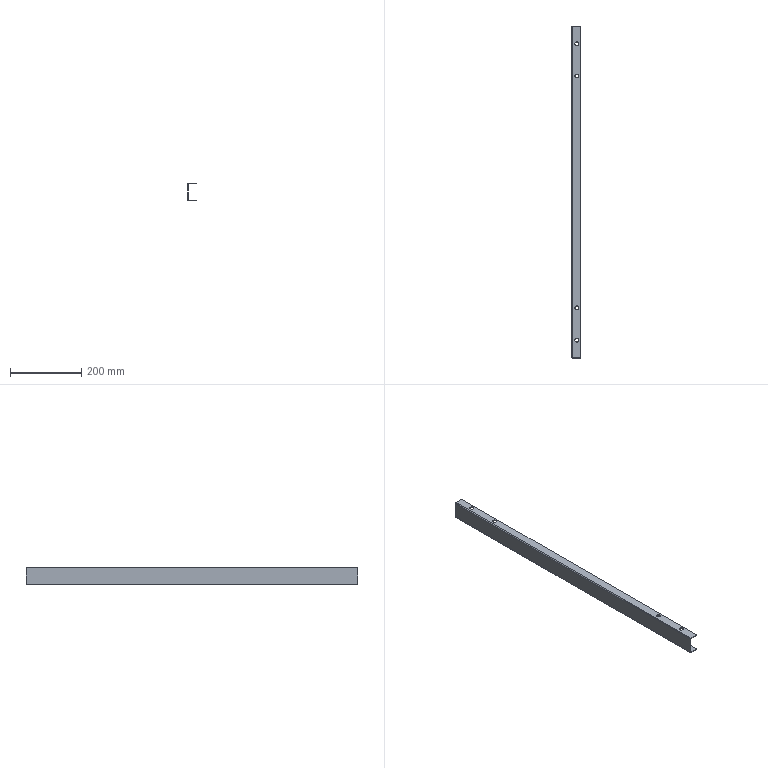Part | 1 solid | 38 faces | box 25 x 929 x 50 mm | volume 174934 mm3 | cylinder 20 | plane 18 | commonest cylinder face diameters 11 x16 0.4 x2 4.4 x2
STEP:
#1=CARTESIAN_POINT('',(20.5,414.5,-23.));
#2=VERTEX_POINT('',#1);
#3=CARTESIAN_POINT('',(9.5,414.5,-23.));
#4=VERTEX_POINT('',#3);
#5=CARTESIAN_POINT('',(15.,414.5,-23.));
#6=DIRECTION('',(0.,0.,-1.));
#7=DIRECTION('',(-1.,0.,0.));
#8=AXIS2_PLACEMENT_3D('',#5,#6,#7);
#9=CIRCLE('',#8,5.5);
#10=EDGE_CURVE('',#2,#4,#9,.T.);
#11=ORIENTED_EDGE('',*,*,#10,.F.);
#12=CARTESIAN_POINT('',(20.5,414.5,-25.));
#13=VERTEX_POINT('',#12);
#14=CARTESIAN_POINT('',(20.5,414.5,25.));
#15=DIRECTION('',(0.,0.,-1.));
#16=VECTOR('',#15,1000.);
#17=LINE('',#14,#16);
#18=EDGE_CURVE('',#2,#13,#17,.T.);
#19=ORIENTED_EDGE('',*,*,#18,.T.);
#20=CARTESIAN_POINT('',(9.5,414.5,-25.));
#21=VERTEX_POINT('',#20);
#22=CARTESIAN_POINT('',(15.,414.5,-25.));
#23=DIRECTION('',(0.,0.,-1.));
#24=DIRECTION('',(-1.,0.,0.));
#25=AXIS2_PLACEMENT_3D('',#22,#23,#24);
#26=CIRCLE('',#25,5.5);
#27=EDGE_CURVE('',#13,#21,#26,.T.);
#28=ORIENTED_EDGE('',*,*,#27,.T.);
#29=CARTESIAN_POINT('',(9.5,414.5,25.));
#30=DIRECTION('',(0.,0.,-1.));
#31=VECTOR('',#30,1000.);
#32=LINE('',#29,#31);
#33=EDGE_CURVE('',#4,#21,#32,.T.);
#34=ORIENTED_EDGE('',*,*,#33,.F.);
#35=EDGE_LOOP('',(#11,#19,#28,#34));
#36=FACE_OUTER_BOUND('',#35,.T.);
#37=CARTESIAN_POINT('',(15.,414.5,25.));
#38=DIRECTION('',(0.,0.,-1.));
#39=DIRECTION('',(-1.,0.,0.));
#40=AXIS2_PLACEMENT_3D('',#37,#38,#39);
#41=CYLINDRICAL_SURFACE('',#40,5.5);
#42=ADVANCED_FACE('',(#36),#41,.F.);
#43=CARTESIAN_POINT('',(20.5,324.5,-23.));
#44=VERTEX_POINT('',#43);
#45=CARTESIAN_POINT('',(9.5,324.5,-23.));
#46=VERTEX_POINT('',#45);
#47=CARTESIAN_POINT('',(15.,324.5,-23.));
#48=DIRECTION('',(0.,0.,-1.));
#49=DIRECTION('',(-1.,0.,0.));
#50=AXIS2_PLACEMENT_3D('',#47,#48,#49);
#51=CIRCLE('',#50,5.5);
#52=EDGE_CURVE('',#44,#46,#51,.T.);
#53=ORIENTED_EDGE('',*,*,#52,.F.);
#54=CARTESIAN_POINT('',(20.5,324.5,-25.));
#55=VERTEX_POINT('',#54);
#56=CARTESIAN_POINT('',(20.5,324.5,25.));
#57=DIRECTION('',(0.,0.,-1.));
#58=VECTOR('',#57,1000.);
#59=LINE('',#56,#58);
#60=EDGE_CURVE('',#44,#55,#59,.T.);
#61=ORIENTED_EDGE('',*,*,#60,.T.);
#62=CARTESIAN_POINT('',(9.5,324.5,-25.));
#63=VERTEX_POINT('',#62);
#64=CARTESIAN_POINT('',(15.,324.5,-25.));
#65=DIRECTION('',(0.,0.,-1.));
#66=DIRECTION('',(-1.,0.,0.));
#67=AXIS2_PLACEMENT_3D('',#64,#65,#66);
#68=CIRCLE('',#67,5.5);
#69=EDGE_CURVE('',#55,#63,#68,.T.);
#70=ORIENTED_EDGE('',*,*,#69,.T.);
#71=CARTESIAN_POINT('',(9.5,324.5,25.));
#72=DIRECTION('',(0.,0.,-1.));
#73=VECTOR('',#72,1000.);
#74=LINE('',#71,#73);
#75=EDGE_CURVE('',#46,#63,#74,.T.);
#76=ORIENTED_EDGE('',*,*,#75,.F.);
#77=EDGE_LOOP('',(#53,#61,#70,#76));
#78=FACE_OUTER_BOUND('',#77,.T.);
#79=CARTESIAN_POINT('',(15.,324.5,25.));
#80=DIRECTION('',(0.,0.,-1.));
#81=DIRECTION('',(-1.,0.,0.));
#82=AXIS2_PLACEMENT_3D('',#79,#80,#81);
#83=CYLINDRICAL_SURFACE('',#82,5.5);
#84=ADVANCED_FACE('',(#78),#83,.F.);
#85=CARTESIAN_POINT('',(20.5,-324.5,-23.));
#86=VERTEX_POINT('',#85);
#87=CARTESIAN_POINT('',(9.5,-324.5,-23.));
#88=VERTEX_POINT('',#87);
#89=CARTESIAN_POINT('',(15.,-324.5,-23.));
#90=DIRECTION('',(0.,0.,-1.));
#91=DIRECTION('',(-1.,0.,0.));
#92=AXIS2_PLACEMENT_3D('',#89,#90,#91);
#93=CIRCLE('',#92,5.5);
#94=EDGE_CURVE('',#86,#88,#93,.T.);
#95=ORIENTED_EDGE('',*,*,#94,.F.);
#96=CARTESIAN_POINT('',(20.5,-324.5,-25.));
#97=VERTEX_POINT('',#96);
#98=CARTESIAN_POINT('',(20.5,-324.5,25.));
#99=DIRECTION('',(0.,0.,-1.));
#100=VECTOR('',#99,1000.);
#101=LINE('',#98,#100);
#102=EDGE_CURVE('',#86,#97,#101,.T.);
#103=ORIENTED_EDGE('',*,*,#102,.T.);
#104=CARTESIAN_POINT('',(9.5,-324.5,-25.));
#105=VERTEX_POINT('',#104);
#106=CARTESIAN_POINT('',(15.,-324.5,-25.));
#107=DIRECTION('',(0.,0.,-1.));
#108=DIRECTION('',(-1.,0.,0.));
#109=AXIS2_PLACEMENT_3D('',#106,#107,#108);
#110=CIRCLE('',#109,5.5);
#111=EDGE_CURVE('',#97,#105,#110,.T.);
#112=ORIENTED_EDGE('',*,*,#111,.T.);
#113=CARTESIAN_POINT('',(9.5,-324.5,25.));
#114=DIRECTION('',(0.,0.,-1.));
#115=VECTOR('',#114,1000.);
#116=LINE('',#113,#115);
#117=EDGE_CURVE('',#88,#105,#116,.T.);
#118=ORIENTED_EDGE('',*,*,#117,.F.);
#119=EDGE_LOOP('',(#95,#103,#112,#118));
#120=FACE_OUTER_BOUND('',#119,.T.);
#121=CARTESIAN_POINT('',(15.,-324.5,25.));
#122=DIRECTION('',(0.,0.,-1.));
#123=DIRECTION('',(-1.,0.,0.));
#124=AXIS2_PLACEMENT_3D('',#121,#122,#123);
#125=CYLINDRICAL_SURFACE('',#124,5.5);
#126=ADVANCED_FACE('',(#120),#125,.F.);
#127=CARTESIAN_POINT('',(20.5,-414.5,-23.));
#128=VERTEX_POINT('',#127);
#129=CARTESIAN_POINT('',(9.5,-414.5,-23.));
#130=VERTEX_POINT('',#129);
#131=CARTESIAN_POINT('',(15.,-414.5,-23.));
#132=DIRECTION('',(0.,0.,-1.));
#133=DIRECTION('',(-1.,0.,0.));
#134=AXIS2_PLACEMENT_3D('',#131,#132,#133);
#135=CIRCLE('',#134,5.5);
#136=EDGE_CURVE('',#128,#130,#135,.T.);
#137=ORIENTED_EDGE('',*,*,#136,.F.);
#138=CARTESIAN_POINT('',(20.5,-414.5,-25.));
#139=VERTEX_POINT('',#138);
#140=CARTESIAN_POINT('',(20.5,-414.5,25.));
#141=DIRECTION('',(0.,0.,-1.));
#142=VECTOR('',#141,1000.);
#143=LINE('',#140,#142);
#144=EDGE_CURVE('',#128,#139,#143,.T.);
#145=ORIENTED_EDGE('',*,*,#144,.T.);
#146=CARTESIAN_POINT('',(9.5,-414.5,-25.));
#147=VERTEX_POINT('',#146);
#148=CARTESIAN_POINT('',(15.,-414.5,-25.));
#149=DIRECTION('',(0.,0.,-1.));
#150=DIRECTION('',(-1.,0.,0.));
#151=AXIS2_PLACEMENT_3D('',#148,#149,#150);
#152=CIRCLE('',#151,5.5);
#153=EDGE_CURVE('',#139,#147,#152,.T.);
#154=ORIENTED_EDGE('',*,*,#153,.T.);
#155=CARTESIAN_POINT('',(9.5,-414.5,25.));
#156=DIRECTION('',(0.,0.,-1.));
#157=VECTOR('',#156,1000.);
#158=LINE('',#155,#157);
#159=EDGE_CURVE('',#130,#147,#158,.T.);
#160=ORIENTED_EDGE('',*,*,#159,.F.);
#161=EDGE_LOOP('',(#137,#145,#154,#160));
#162=FACE_OUTER_BOUND('',#161,.T.);
#163=CARTESIAN_POINT('',(15.,-414.5,25.));
#164=DIRECTION('',(0.,0.,-1.));
#165=DIRECTION('',(-1.,0.,0.));
#166=AXIS2_PLACEMENT_3D('',#163,#164,#165);
#167=CYLINDRICAL_SURFACE('',#166,5.5);
#168=ADVANCED_FACE('',(#162),#167,.F.);
#169=CARTESIAN_POINT('',(20.5,414.5,25.));
#170=VERTEX_POINT('',#169);
#171=CARTESIAN_POINT('',(9.5,414.5,25.));
#172=VERTEX_POINT('',#171);
#173=CARTESIAN_POINT('',(15.,414.5,25.));
#174=DIRECTION('',(0.,0.,-1.));
#175=DIRECTION('',(-1.,0.,0.));
#176=AXIS2_PLACEMENT_3D('',#173,#174,#175);
#177=CIRCLE('',#176,5.5);
#178=EDGE_CURVE('',#170,#172,#177,.T.);
#179=ORIENTED_EDGE('',*,*,#178,.F.);
#180=CARTESIAN_POINT('',(20.5,414.5,23.));
#181=VERTEX_POINT('',#180);
#182=CARTESIAN_POINT('',(20.5,414.5,25.));
#183=DIRECTION('',(0.,0.,-1.));
#184=VECTOR('',#183,1000.);
#185=LINE('',#182,#184);
#186=EDGE_CURVE('',#170,#181,#185,.T.);
#187=ORIENTED_EDGE('',*,*,#186,.T.);
#188=CARTESIAN_POINT('',(9.5,414.5,23.));
#189=VERTEX_POINT('',#188);
#190=CARTESIAN_POINT('',(15.,414.5,23.));
#191=DIRECTION('',(0.,0.,1.));
#192=DIRECTION('',(1.,0.,0.));
#193=AXIS2_PLACEMENT_3D('',#190,#191,#192);
#194=CIRCLE('',#193,5.5);
#195=EDGE_CURVE('',#189,#181,#194,.T.);
#196=ORIENTED_EDGE('',*,*,#195,.F.);
#197=CARTESIAN_POINT('',(9.5,414.5,25.));
#198=DIRECTION('',(0.,0.,-1.));
#199=VECTOR('',#198,1000.);
#200=LINE('',#197,#199);
#201=EDGE_CURVE('',#172,#189,#200,.T.);
#202=ORIENTED_EDGE('',*,*,#201,.F.);
#203=EDGE_LOOP('',(#179,#187,#196,#202));
#204=FACE_OUTER_BOUND('',#203,.T.);
#205=CARTESIAN_POINT('',(15.,414.5,25.));
#206=DIRECTION('',(0.,0.,-1.));
#207=DIRECTION('',(-1.,0.,0.));
#208=AXIS2_PLACEMENT_3D('',#205,#206,#207);
#209=CYLINDRICAL_SURFACE('',#208,5.5);
#210=ADVANCED_FACE('',(#204),#209,.F.);
#211=CARTESIAN_POINT('',(20.5,324.5,25.));
#212=VERTEX_POINT('',#211);
#213=CARTESIAN_POINT('',(9.5,324.5,25.));
#214=VERTEX_POINT('',#213);
#215=CARTESIAN_POINT('',(15.,324.5,25.));
#216=DIRECTION('',(0.,0.,-1.));
#217=DIRECTION('',(-1.,0.,0.));
#218=AXIS2_PLACEMENT_3D('',#215,#216,#217);
#219=CIRCLE('',#218,5.5);
#220=EDGE_CURVE('',#212,#214,#219,.T.);
#221=ORIENTED_EDGE('',*,*,#220,.F.);
#222=CARTESIAN_POINT('',(20.5,324.5,23.));
#223=VERTEX_POINT('',#222);
#224=CARTESIAN_POINT('',(20.5,324.5,25.));
#225=DIRECTION('',(0.,0.,-1.));
#226=VECTOR('',#225,1000.);
#227=LINE('',#224,#226);
#228=EDGE_CURVE('',#212,#223,#227,.T.);
#229=ORIENTED_EDGE('',*,*,#228,.T.);
#230=CARTESIAN_POINT('',(9.5,324.5,23.));
#231=VERTEX_POINT('',#230);
#232=CARTESIAN_POINT('',(15.,324.5,23.));
#233=DIRECTION('',(0.,0.,1.));
#234=DIRECTION('',(1.,0.,0.));
#235=AXIS2_PLACEMENT_3D('',#232,#233,#234);
#236=CIRCLE('',#235,5.5);
#237=EDGE_CURVE('',#231,#223,#236,.T.);
#238=ORIENTED_EDGE('',*,*,#237,.F.);
#239=CARTESIAN_POINT('',(9.5,324.5,25.));
#240=DIRECTION('',(0.,0.,-1.));
#241=VECTOR('',#240,1000.);
#242=LINE('',#239,#241);
#243=EDGE_CURVE('',#214,#231,#242,.T.);
#244=ORIENTED_EDGE('',*,*,#243,.F.);
#245=EDGE_LOOP('',(#221,#229,#238,#244));
#246=FACE_OUTER_BOUND('',#245,.T.);
#247=CARTESIAN_POINT('',(15.,324.5,25.));
#248=DIRECTION('',(0.,0.,-1.));
#249=DIRECTION('',(-1.,0.,0.));
#250=AXIS2_PLACEMENT_3D('',#247,#248,#249);
#251=CYLINDRICAL_SURFACE('',#250,5.5);
#252=ADVANCED_FACE('',(#246),#251,.F.);
#253=CARTESIAN_POINT('',(20.5,-324.5,25.));
#254=VERTEX_POINT('',#253);
#255=CARTESIAN_POINT('',(9.5,-324.5,25.));
#256=VERTEX_POINT('',#255);
#257=CARTESIAN_POINT('',(15.,-324.5,25.));
#258=DIRECTION('',(0.,0.,-1.));
#259=DIRECTION('',(1.,0.,0.));
#260=AXIS2_PLACEMENT_3D('',#257,#258,#259);
#261=CIRCLE('',#260,5.5);
#262=EDGE_CURVE('',#254,#256,#261,.T.);
#263=ORIENTED_EDGE('',*,*,#262,.F.);
#264=CARTESIAN_POINT('',(20.5,-324.5,23.));
#265=VERTEX_POINT('',#264);
#266=CARTESIAN_POINT('',(20.5,-324.5,25.));
#267=DIRECTION('',(0.,0.,-1.));
#268=VECTOR('',#267,1000.);
#269=LINE('',#266,#268);
#270=EDGE_CURVE('',#254,#265,#269,.T.);
#271=ORIENTED_EDGE('',*,*,#270,.T.);
#272=CARTESIAN_POINT('',(9.5,-324.5,23.));
#273=VERTEX_POINT('',#272);
#274=CARTESIAN_POINT('',(15.,-324.5,23.));
#275=DIRECTION('',(0.,0.,1.));
#276=DIRECTION('',(1.,0.,0.));
#277=AXIS2_PLACEMENT_3D('',#274,#275,#276);
#278=CIRCLE('',#277,5.5);
#279=EDGE_CURVE('',#273,#265,#278,.T.);
#280=ORIENTED_EDGE('',*,*,#279,.F.);
#281=CARTESIAN_POINT('',(9.5,-324.5,25.));
#282=DIRECTION('',(0.,0.,-1.));
#283=VECTOR('',#282,1000.);
#284=LINE('',#281,#283);
#285=EDGE_CURVE('',#256,#273,#284,.T.);
#286=ORIENTED_EDGE('',*,*,#285,.F.);
#287=EDGE_LOOP('',(#263,#271,#280,#286));
#288=FACE_OUTER_BOUND('',#287,.T.);
#289=CARTESIAN_POINT('',(15.,-324.5,25.));
#290=DIRECTION('',(0.,0.,-1.));
#291=DIRECTION('',(-1.,0.,0.));
#292=AXIS2_PLACEMENT_3D('',#289,#290,#291);
#293=CYLINDRICAL_SURFACE('',#292,5.5);
#294=ADVANCED_FACE('',(#288),#293,.F.);
#295=CARTESIAN_POINT('',(20.5,-414.5,25.));
#296=VERTEX_POINT('',#295);
#297=CARTESIAN_POINT('',(9.5,-414.5,25.));
#298=VERTEX_POINT('',#297);
#299=CARTESIAN_POINT('',(15.,-414.5,25.));
#300=DIRECTION('',(0.,0.,-1.));
#301=DIRECTION('',(1.,0.,0.));
#302=AXIS2_PLACEMENT_3D('',#299,#300,#301);
#303=CIRCLE('',#302,5.5);
#304=EDGE_CURVE('',#296,#298,#303,.T.);
#305=ORIENTED_EDGE('',*,*,#304,.F.);
#306=CARTESIAN_POINT('',(20.5,-414.5,23.));
#307=VERTEX_POINT('',#306);
#308=CARTESIAN_POINT('',(20.5,-414.5,25.));
#309=DIRECTION('',(0.,0.,-1.));
#310=VECTOR('',#309,1000.);
#311=LINE('',#308,#310);
#312=EDGE_CURVE('',#296,#307,#311,.T.);
#313=ORIENTED_EDGE('',*,*,#312,.T.);
#314=CARTESIAN_POINT('',(9.5,-414.5,23.));
#315=VERTEX_POINT('',#314);
#316=CARTESIAN_POINT('',(15.,-414.5,23.));
#317=DIRECTION('',(0.,0.,1.));
#318=DIRECTION('',(1.,0.,0.));
#319=AXIS2_PLACEMENT_3D('',#316,#317,#318);
#320=CIRCLE('',#319,5.5);
#321=EDGE_CURVE('',#315,#307,#320,.T.);
#322=ORIENTED_EDGE('',*,*,#321,.F.);
#323=CARTESIAN_POINT('',(9.5,-414.5,25.));
#324=DIRECTION('',(0.,0.,-1.));
#325=VECTOR('',#324,1000.);
#326=LINE('',#323,#325);
#327=EDGE_CURVE('',#298,#315,#326,.T.);
#328=ORIENTED_EDGE('',*,*,#327,.F.);
#329=EDGE_LOOP('',(#305,#313,#322,#328));
#330=FACE_OUTER_BOUND('',#329,.T.);
#331=CARTESIAN_POINT('',(15.,-414.5,25.));
#332=DIRECTION('',(0.,0.,-1.));
#333=DIRECTION('',(-1.,0.,0.));
#334=AXIS2_PLACEMENT_3D('',#331,#332,#333);
#335=CYLINDRICAL_SURFACE('',#334,5.5);
#336=ADVANCED_FACE('',(#330),#335,.F.);
#337=CARTESIAN_POINT('',(0.,464.5,22.8));
#338=VERTEX_POINT('',#337);
#339=CARTESIAN_POINT('',(2.,464.5,22.8));
#340=VERTEX_POINT('',#339);
#341=CARTESIAN_POINT('',(0.,464.5,22.8));
#342=DIRECTION('',(1.,0.,0.));
#343=VECTOR('',#342,1000.);
#344=LINE('',#341,#343);
#345=EDGE_CURVE('',#338,#340,#344,.T.);
#346=ORIENTED_EDGE('',*,*,#345,.F.);
#347=CARTESIAN_POINT('',(2.2,464.5,25.));
#348=VERTEX_POINT('',#347);
#349=CARTESIAN_POINT('',(2.2,464.5,22.8));
#350=DIRECTION('',(0.,-1.,0.));
#351=DIRECTION('',(0.,0.,1.));
#352=AXIS2_PLACEMENT_3D('',#349,#350,#351);
#353=CIRCLE('',#352,2.2);
#354=EDGE_CURVE('',#348,#338,#353,.T.);
#355=ORIENTED_EDGE('',*,*,#354,.F.);
#356=CARTESIAN_POINT('',(2.2,464.5,23.));
#357=VERTEX_POINT('',#356);
#358=CARTESIAN_POINT('',(2.2,464.5,23.));
#359=DIRECTION('',(0.,0.,1.));
#360=VECTOR('',#359,1000.);
#361=LINE('',#358,#360);
#362=EDGE_CURVE('',#357,#348,#361,.T.);
#363=ORIENTED_EDGE('',*,*,#362,.F.);
#364=CARTESIAN_POINT('',(2.2,464.5,22.8));
#365=DIRECTION('',(0.,-1.,0.));
#366=DIRECTION('',(1.,0.,0.));
#367=AXIS2_PLACEMENT_3D('',#364,#365,#366);
#368=CIRCLE('',#367,0.2);
#369=EDGE_CURVE('',#357,#340,#368,.T.);
#370=ORIENTED_EDGE('',*,*,#369,.T.);
#371=EDGE_LOOP('',(#346,#355,#363,#370));
#372=FACE_OUTER_BOUND('',#371,.T.);
#373=CARTESIAN_POINT('',(0.,464.5,22.8));
#374=DIRECTION('',(0.,1.,0.));
#375=DIRECTION('',(0.,0.,1.));
#376=AXIS2_PLACEMENT_3D('',#373,#374,#375);
#377=PLANE('',#376);
#378=ADVANCED_FACE('',(#372),#377,.T.);
#379=CARTESIAN_POINT('',(0.,464.5,-22.8));
#380=VERTEX_POINT('',#379);
#381=CARTESIAN_POINT('',(0.,464.5,-25.));
#382=DIRECTION('',(0.,0.,-1.));
#383=VECTOR('',#382,1000.);
#384=LINE('',#381,#383);
#385=EDGE_CURVE('',#338,#380,#384,.T.);
#386=ORIENTED_EDGE('',*,*,#385,.F.);
#387=ORIENTED_EDGE('',*,*,#345,.T.);
#388=CARTESIAN_POINT('',(2.,464.5,-22.8));
#389=VERTEX_POINT('',#388);
#390=CARTESIAN_POINT('',(2.,464.5,-25.));
#391=DIRECTION('',(0.,0.,-1.));
#392=VECTOR('',#391,1000.);
#393=LINE('',#390,#392);
#394=EDGE_CURVE('',#340,#389,#393,.T.);
#395=ORIENTED_EDGE('',*,*,#394,.T.);
#396=CARTESIAN_POINT('',(2.,464.5,-22.8));
#397=DIRECTION('',(-1.,0.,0.));
#398=VECTOR('',#397,1000.);
#399=LINE('',#396,#398);
#400=EDGE_CURVE('',#389,#380,#399,.T.);
#401=ORIENTED_EDGE('',*,*,#400,.T.);
#402=EDGE_LOOP('',(#386,#387,#395,#401));
#403=FACE_OUTER_BOUND('',#402,.T.);
#404=CARTESIAN_POINT('',(2.2,464.5,23.));
#405=DIRECTION('',(0.,1.,0.));
#406=DIRECTION('',(0.,0.,1.));
#407=AXIS2_PLACEMENT_3D('',#404,#405,#406);
#408=PLANE('',#407);
#409=ADVANCED_FACE('',(#403),#408,.T.);
#410=CARTESIAN_POINT('',(2.2,-464.5,25.));
#411=VERTEX_POINT('',#410);
#412=CARTESIAN_POINT('',(2.2,-464.5,23.));
#413=VERTEX_POINT('',#412);
#414=CARTESIAN_POINT('',(2.2,-464.5,25.));
#415=DIRECTION('',(0.,0.,-1.));
#416=VECTOR('',#415,1000.);
#417=LINE('',#414,#416);
#418=EDGE_CURVE('',#411,#413,#417,.T.);
#419=ORIENTED_EDGE('',*,*,#418,.F.);
#420=CARTESIAN_POINT('',(0.,-464.5,22.8));
#421=VERTEX_POINT('',#420);
#422=CARTESIAN_POINT('',(2.2,-464.5,22.8));
#423=DIRECTION('',(0.,-1.,0.));
#424=DIRECTION('',(0.,0.,1.));
#425=AXIS2_PLACEMENT_3D('',#422,#423,#424);
#426=CIRCLE('',#425,2.2);
#427=EDGE_CURVE('',#411,#421,#426,.T.);
#428=ORIENTED_EDGE('',*,*,#427,.T.);
#429=CARTESIAN_POINT('',(2.,-464.5,22.8));
#430=VERTEX_POINT('',#429);
#431=CARTESIAN_POINT('',(2.,-464.5,22.8));
#432=DIRECTION('',(-1.,0.,0.));
#433=VECTOR('',#432,1000.);
#434=LINE('',#431,#433);
#435=EDGE_CURVE('',#430,#421,#434,.T.);
#436=ORIENTED_EDGE('',*,*,#435,.F.);
#437=CARTESIAN_POINT('',(2.2,-464.5,22.8));
#438=DIRECTION('',(0.,-1.,0.));
#439=DIRECTION('',(1.,0.,0.));
#440=AXIS2_PLACEMENT_3D('',#437,#438,#439);
#441=CIRCLE('',#440,0.2);
#442=EDGE_CURVE('',#413,#430,#441,.T.);
#443=ORIENTED_EDGE('',*,*,#442,.F.);
#444=EDGE_LOOP('',(#419,#428,#436,#443));
#445=FACE_OUTER_BOUND('',#444,.T.);
#446=CARTESIAN_POINT('',(2.2,-464.5,25.));
#447=DIRECTION('',(0.,-1.,0.));
#448=DIRECTION('',(0.,0.,-1.));
#449=AXIS2_PLACEMENT_3D('',#446,#447,#448);
#450=PLANE('',#449);
#451=ADVANCED_FACE('',(#445),#450,.T.);
#452=CARTESIAN_POINT('',(25.,-464.5,25.));
#453=VERTEX_POINT('',#452);
#454=CARTESIAN_POINT('',(0.,-464.5,25.));
#455=DIRECTION('',(-1.,0.,0.));
#456=VECTOR('',#455,1000.);
#457=LINE('',#454,#456);
#458=EDGE_CURVE('',#453,#411,#457,.T.);
#459=ORIENTED_EDGE('',*,*,#458,.T.);
#460=ORIENTED_EDGE('',*,*,#418,.T.);
#461=CARTESIAN_POINT('',(25.,-464.5,23.));
#462=VERTEX_POINT('',#461);
#463=CARTESIAN_POINT('',(0.,-464.5,23.));
#464=DIRECTION('',(-1.,0.,0.));
#465=VECTOR('',#464,1000.);
#466=LINE('',#463,#465);
#467=EDGE_CURVE('',#462,#413,#466,.T.);
#468=ORIENTED_EDGE('',*,*,#467,.F.);
#469=CARTESIAN_POINT('',(25.,-464.5,23.));
#470=DIRECTION('',(0.,0.,1.));
#471=VECTOR('',#470,1000.);
#472=LINE('',#469,#471);
#473=EDGE_CURVE('',#462,#453,#472,.T.);
#474=ORIENTED_EDGE('',*,*,#473,.T.);
#475=EDGE_LOOP('',(#459,#460,#468,#474));
#476=FACE_OUTER_BOUND('',#475,.T.);
#477=CARTESIAN_POINT('',(2.,-464.5,22.8));
#478=DIRECTION('',(0.,-1.,0.));
#479=DIRECTION('',(0.,0.,-1.));
#480=AXIS2_PLACEMENT_3D('',#477,#478,#479);
#481=PLANE('',#480);
#482=ADVANCED_FACE('',(#476),#481,.T.);
#483=CARTESIAN_POINT('',(2.2,464.5,-25.));
#484=VERTEX_POINT('',#483);
#485=CARTESIAN_POINT('',(2.2,464.5,-23.));
#486=VERTEX_POINT('',#485);
#487=CARTESIAN_POINT('',(2.2,464.5,-25.));
#488=DIRECTION('',(0.,0.,1.));
#489=VECTOR('',#488,1000.);
#490=LINE('',#487,#489);
#491=EDGE_CURVE('',#484,#486,#490,.T.);
#492=ORIENTED_EDGE('',*,*,#491,.F.);
#493=CARTESIAN_POINT('',(2.2,464.5,-22.8));
#494=DIRECTION('',(0.,-1.,0.));
#495=DIRECTION('',(0.,0.,1.));
#496=AXIS2_PLACEMENT_3D('',#493,#494,#495);
#497=CIRCLE('',#496,2.2);
#498=EDGE_CURVE('',#380,#484,#497,.T.);
#499=ORIENTED_EDGE('',*,*,#498,.F.);
#500=ORIENTED_EDGE('',*,*,#400,.F.);
#501=CARTESIAN_POINT('',(2.2,464.5,-22.8));
#502=DIRECTION('',(0.,-1.,0.));
#503=DIRECTION('',(1.,0.,0.));
#504=AXIS2_PLACEMENT_3D('',#501,#502,#503);
#505=CIRCLE('',#504,0.2);
#506=EDGE_CURVE('',#389,#486,#505,.T.);
#507=ORIENTED_EDGE('',*,*,#506,.T.);
#508=EDGE_LOOP('',(#492,#499,#500,#507));
#509=FACE_OUTER_BOUND('',#508,.T.);
#510=CARTESIAN_POINT('',(2.2,464.5,-25.));
#511=DIRECTION('',(0.,1.,0.));
#512=DIRECTION('',(0.,0.,1.));
#513=AXIS2_PLACEMENT_3D('',#510,#511,#512);
#514=PLANE('',#513);
#515=ADVANCED_FACE('',(#509),#514,.T.);
#516=CARTESIAN_POINT('',(25.,464.5,-25.));
#517=VERTEX_POINT('',#516);
#518=CARTESIAN_POINT('',(0.,464.5,-25.));
#519=DIRECTION('',(1.,0.,0.));
#520=VECTOR('',#519,1000.);
#521=LINE('',#518,#520);
#522=EDGE_CURVE('',#484,#517,#521,.T.);
#523=ORIENTED_EDGE('',*,*,#522,.F.);
#524=ORIENTED_EDGE('',*,*,#491,.T.);
#525=CARTESIAN_POINT('',(25.,464.5,-23.));
#526=VERTEX_POINT('',#525);
#527=CARTESIAN_POINT('',(0.,464.5,-23.));
#528=DIRECTION('',(1.,0.,0.));
#529=VECTOR('',#528,1000.);
#530=LINE('',#527,#529);
#531=EDGE_CURVE('',#486,#526,#530,.T.);
#532=ORIENTED_EDGE('',*,*,#531,.T.);
#533=CARTESIAN_POINT('',(25.,464.5,-25.));
#534=DIRECTION('',(0.,0.,1.));
#535=VECTOR('',#534,1000.);
#536=LINE('',#533,#535);
#537=EDGE_CURVE('',#517,#526,#536,.T.);
#538=ORIENTED_EDGE('',*,*,#537,.F.);
#539=EDGE_LOOP('',(#523,#524,#532,#538));
#540=FACE_OUTER_BOUND('',#539,.T.);
#541=CARTESIAN_POINT('',(2.,464.5,-22.8));
#542=DIRECTION('',(0.,1.,0.));
#543=DIRECTION('',(0.,0.,1.));
#544=AXIS2_PLACEMENT_3D('',#541,#542,#543);
#545=PLANE('',#544);
#546=ADVANCED_FACE('',(#540),#545,.T.);
#547=CARTESIAN_POINT('',(0.,-464.5,-22.8));
#548=VERTEX_POINT('',#547);
#549=CARTESIAN_POINT('',(2.,-464.5,-22.8));
#550=VERTEX_POINT('',#549);
#551=CARTESIAN_POINT('',(0.,-464.5,-22.8));
#552=DIRECTION('',(1.,0.,0.));
#553=VECTOR('',#552,1000.);
#554=LINE('',#551,#553);
#555=EDGE_CURVE('',#548,#550,#554,.T.);
#556=ORIENTED_EDGE('',*,*,#555,.F.);
#557=CARTESIAN_POINT('',(2.2,-464.5,-25.));
#558=VERTEX_POINT('',#557);
#559=CARTESIAN_POINT('',(2.2,-464.5,-22.8));
#560=DIRECTION('',(0.,-1.,0.));
#561=DIRECTION('',(0.,0.,1.));
#562=AXIS2_PLACEMENT_3D('',#559,#560,#561);
#563=CIRCLE('',#562,2.2);
#564=EDGE_CURVE('',#548,#558,#563,.T.);
#565=ORIENTED_EDGE('',*,*,#564,.T.);
#566=CARTESIAN_POINT('',(2.2,-464.5,-23.));
#567=VERTEX_POINT('',#566);
#568=CARTESIAN_POINT('',(2.2,-464.5,-23.));
#569=DIRECTION('',(0.,0.,-1.));
#570=VECTOR('',#569,1000.);
#571=LINE('',#568,#570);
#572=EDGE_CURVE('',#567,#558,#571,.T.);
#573=ORIENTED_EDGE('',*,*,#572,.F.);
#574=CARTESIAN_POINT('',(2.2,-464.5,-22.8));
#575=DIRECTION('',(0.,-1.,0.));
#576=DIRECTION('',(1.,0.,0.));
#577=AXIS2_PLACEMENT_3D('',#574,#575,#576);
#578=CIRCLE('',#577,0.2);
#579=EDGE_CURVE('',#550,#567,#578,.T.);
#580=ORIENTED_EDGE('',*,*,#579,.F.);
#581=EDGE_LOOP('',(#556,#565,#573,#580));
#582=FACE_OUTER_BOUND('',#581,.T.);
#583=CARTESIAN_POINT('',(0.,-464.5,-22.8));
#584=DIRECTION('',(0.,-1.,0.));
#585=DIRECTION('',(0.,0.,-1.));
#586=AXIS2_PLACEMENT_3D('',#583,#584,#585);
#587=PLANE('',#586);
#588=ADVANCED_FACE('',(#582),#587,.T.);
#589=CARTESIAN_POINT('',(0.,-464.5,-25.));
#590=DIRECTION('',(0.,0.,-1.));
#591=VECTOR('',#590,1000.);
#592=LINE('',#589,#591);
#593=EDGE_CURVE('',#421,#548,#592,.T.);
#594=ORIENTED_EDGE('',*,*,#593,.T.);
#595=ORIENTED_EDGE('',*,*,#555,.T.);
#596=CARTESIAN_POINT('',(2.,-464.5,-25.));
#597=DIRECTION('',(0.,0.,-1.));
#598=VECTOR('',#597,1000.);
#599=LINE('',#596,#598);
#600=EDGE_CURVE('',#430,#550,#599,.T.);
#601=ORIENTED_EDGE('',*,*,#600,.F.);
#602=ORIENTED_EDGE('',*,*,#435,.T.);
#603=EDGE_LOOP('',(#594,#595,#601,#602));
#604=FACE_OUTER_BOUND('',#603,.T.);
#605=CARTESIAN_POINT('',(2.2,-464.5,-23.));
#606=DIRECTION('',(0.,-1.,0.));
#607=DIRECTION('',(0.,0.,-1.));
#608=AXIS2_PLACEMENT_3D('',#605,#606,#607);
#609=PLANE('',#608);
#610=ADVANCED_FACE('',(#604),#609,.T.);
#611=CARTESIAN_POINT('',(15.,414.5,-23.));
#612=DIRECTION('',(0.,0.,-1.));
#613=DIRECTION('',(-1.,0.,0.));
#614=AXIS2_PLACEMENT_3D('',#611,#612,#613);
#615=CIRCLE('',#614,5.5);
#616=EDGE_CURVE('',#4,#2,#615,.T.);
#617=ORIENTED_EDGE('',*,*,#616,.T.);
#618=ORIENTED_EDGE('',*,*,#10,.T.);
#619=EDGE_LOOP('',(#617,#618));
#620=FACE_BOUND('',#619,.T.);
#621=CARTESIAN_POINT('',(15.,324.5,-23.));
#622=DIRECTION('',(0.,0.,-1.));
#623=DIRECTION('',(-1.,0.,0.));
#624=AXIS2_PLACEMENT_3D('',#621,#622,#623);
#625=CIRCLE('',#624,5.5);
#626=EDGE_CURVE('',#46,#44,#625,.T.);
#627=ORIENTED_EDGE('',*,*,#626,.T.);
#628=ORIENTED_EDGE('',*,*,#52,.T.);
#629=EDGE_LOOP('',(#627,#628));
#630=FACE_BOUND('',#629,.T.);
#631=CARTESIAN_POINT('',(15.,-324.5,-23.));
#632=DIRECTION('',(0.,0.,-1.));
#633=DIRECTION('',(-1.,0.,0.));
#634=AXIS2_PLACEMENT_3D('',#631,#632,#633);
#635=CIRCLE('',#634,5.5);
#636=EDGE_CURVE('',#88,#86,#635,.T.);
#637=ORIENTED_EDGE('',*,*,#636,.T.);
#638=ORIENTED_EDGE('',*,*,#94,.T.);
#639=EDGE_LOOP('',(#637,#638));
#640=FACE_BOUND('',#639,.T.);
#641=CARTESIAN_POINT('',(15.,-414.5,-23.));
#642=DIRECTION('',(0.,0.,-1.));
#643=DIRECTION('',(-1.,0.,0.));
#644=AXIS2_PLACEMENT_3D('',#641,#642,#643);
#645=CIRCLE('',#644,5.5);
#646=EDGE_CURVE('',#130,#128,#645,.T.);
#647=ORIENTED_EDGE('',*,*,#646,.T.);
#648=ORIENTED_EDGE('',*,*,#136,.T.);
#649=EDGE_LOOP('',(#647,#648));
#650=FACE_BOUND('',#649,.T.);
#651=CARTESIAN_POINT('',(25.,-464.5,-23.));
#652=VERTEX_POINT('',#651);
#653=CARTESIAN_POINT('',(0.,-464.5,-23.));
#654=DIRECTION('',(1.,0.,0.));
#655=VECTOR('',#654,1000.);
#656=LINE('',#653,#655);
#657=EDGE_CURVE('',#567,#652,#656,.T.);
#658=ORIENTED_EDGE('',*,*,#657,.T.);
#659=CARTESIAN_POINT('',(25.,464.5,-23.));
#660=DIRECTION('',(0.,-1.,0.));
#661=VECTOR('',#660,1000.);
#662=LINE('',#659,#661);
#663=EDGE_CURVE('',#526,#652,#662,.T.);
#664=ORIENTED_EDGE('',*,*,#663,.F.);
#665=ORIENTED_EDGE('',*,*,#531,.F.);
#666=CARTESIAN_POINT('',(2.2,464.5,-23.));
#667=DIRECTION('',(0.,-1.,0.));
#668=VECTOR('',#667,1000.);
#669=LINE('',#666,#668);
#670=EDGE_CURVE('',#486,#567,#669,.T.);
#671=ORIENTED_EDGE('',*,*,#670,.T.);
#672=EDGE_LOOP('',(#658,#664,#665,#671));
#673=FACE_OUTER_BOUND('',#672,.T.);
#674=CARTESIAN_POINT('',(0.,464.5,-23.));
#675=DIRECTION('',(0.,0.,-1.));
#676=DIRECTION('',(-1.,0.,0.));
#677=AXIS2_PLACEMENT_3D('',#674,#675,#676);
#678=PLANE('',#677);
#679=ADVANCED_FACE('',(#620,#630,#640,#650,#673),#678,.F.);
#680=CARTESIAN_POINT('',(25.,-464.5,-25.));
#681=VERTEX_POINT('',#680);
#682=CARTESIAN_POINT('',(25.,-464.5,-25.));
#683=DIRECTION('',(0.,0.,1.));
#684=VECTOR('',#683,1000.);
#685=LINE('',#682,#684);
#686=EDGE_CURVE('',#681,#652,#685,.T.);
#687=ORIENTED_EDGE('',*,*,#686,.F.);
#688=CARTESIAN_POINT('',(25.,464.5,-25.));
#689=DIRECTION('',(0.,-1.,0.));
#690=VECTOR('',#689,1000.);
#691=LINE('',#688,#690);
#692=EDGE_CURVE('',#517,#681,#691,.T.);
#693=ORIENTED_EDGE('',*,*,#692,.F.);
#694=ORIENTED_EDGE('',*,*,#537,.T.);
#695=ORIENTED_EDGE('',*,*,#663,.T.);
#696=EDGE_LOOP('',(#687,#693,#694,#695));
#697=FACE_OUTER_BOUND('',#696,.T.);
#698=CARTESIAN_POINT('',(25.,464.5,-25.));
#699=DIRECTION('',(1.,0.,0.));
#700=DIRECTION('',(0.,0.,-1.));
#701=AXIS2_PLACEMENT_3D('',#698,#699,#700);
#702=PLANE('',#701);
#703=ADVANCED_FACE('',(#697),#702,.T.);
#704=CARTESIAN_POINT('',(15.,414.5,-25.));
#705=DIRECTION('',(0.,0.,-1.));
#706=DIRECTION('',(-1.,0.,0.));
#707=AXIS2_PLACEMENT_3D('',#704,#705,#706);
#708=CIRCLE('',#707,5.5);
#709=EDGE_CURVE('',#21,#13,#708,.T.);
#710=ORIENTED_EDGE('',*,*,#709,.F.);
#711=ORIENTED_EDGE('',*,*,#27,.F.);
#712=EDGE_LOOP('',(#710,#711));
#713=FACE_BOUND('',#712,.T.);
#714=CARTESIAN_POINT('',(15.,324.5,-25.));
#715=DIRECTION('',(0.,0.,-1.));
#716=DIRECTION('',(-1.,0.,0.));
#717=AXIS2_PLACEMENT_3D('',#714,#715,#716);
#718=CIRCLE('',#717,5.5);
#719=EDGE_CURVE('',#63,#55,#718,.T.);
#720=ORIENTED_EDGE('',*,*,#719,.F.);
#721=ORIENTED_EDGE('',*,*,#69,.F.);
#722=EDGE_LOOP('',(#720,#721));
#723=FACE_BOUND('',#722,.T.);
#724=CARTESIAN_POINT('',(15.,-324.5,-25.));
#725=DIRECTION('',(0.,0.,-1.));
#726=DIRECTION('',(-1.,0.,0.));
#727=AXIS2_PLACEMENT_3D('',#724,#725,#726);
#728=CIRCLE('',#727,5.5);
#729=EDGE_CURVE('',#105,#97,#728,.T.);
#730=ORIENTED_EDGE('',*,*,#729,.F.);
#731=ORIENTED_EDGE('',*,*,#111,.F.);
#732=EDGE_LOOP('',(#730,#731));
#733=FACE_BOUND('',#732,.T.);
#734=CARTESIAN_POINT('',(15.,-414.5,-25.));
#735=DIRECTION('',(0.,0.,-1.));
#736=DIRECTION('',(-1.,0.,0.));
#737=AXIS2_PLACEMENT_3D('',#734,#735,#736);
#738=CIRCLE('',#737,5.5);
#739=EDGE_CURVE('',#147,#139,#738,.T.);
#740=ORIENTED_EDGE('',*,*,#739,.F.);
#741=ORIENTED_EDGE('',*,*,#153,.F.);
#742=EDGE_LOOP('',(#740,#741));
#743=FACE_BOUND('',#742,.T.);
#744=CARTESIAN_POINT('',(0.,-464.5,-25.));
#745=DIRECTION('',(1.,0.,0.));
#746=VECTOR('',#745,1000.);
#747=LINE('',#744,#746);
#748=EDGE_CURVE('',#558,#681,#747,.T.);
#749=ORIENTED_EDGE('',*,*,#748,.F.);
#750=CARTESIAN_POINT('',(2.2,464.5,-25.));
#751=DIRECTION('',(0.,-1.,0.));
#752=VECTOR('',#751,1000.);
#753=LINE('',#750,#752);
#754=EDGE_CURVE('',#484,#558,#753,.T.);
#755=ORIENTED_EDGE('',*,*,#754,.F.);
#756=ORIENTED_EDGE('',*,*,#522,.T.);
#757=ORIENTED_EDGE('',*,*,#692,.T.);
#758=EDGE_LOOP('',(#749,#755,#756,#757));
#759=FACE_OUTER_BOUND('',#758,.T.);
#760=CARTESIAN_POINT('',(0.,464.5,-25.));
#761=DIRECTION('',(0.,0.,-1.));
#762=DIRECTION('',(-1.,0.,0.));
#763=AXIS2_PLACEMENT_3D('',#760,#761,#762);
#764=PLANE('',#763);
#765=ADVANCED_FACE('',(#713,#723,#733,#743,#759),#764,.T.);
#766=ORIENTED_EDGE('',*,*,#564,.F.);
#767=CARTESIAN_POINT('',(0.,464.5,-22.8));
#768=DIRECTION('',(0.,-1.,0.));
#769=VECTOR('',#768,1000.);
#770=LINE('',#767,#769);
#771=EDGE_CURVE('',#380,#548,#770,.T.);
#772=ORIENTED_EDGE('',*,*,#771,.F.);
#773=ORIENTED_EDGE('',*,*,#498,.T.);
#774=ORIENTED_EDGE('',*,*,#754,.T.);
#775=EDGE_LOOP('',(#766,#772,#773,#774));
#776=FACE_OUTER_BOUND('',#775,.T.);
#777=CARTESIAN_POINT('',(2.2,464.5,-22.8));
#778=DIRECTION('',(0.,-1.,0.));
#779=DIRECTION('',(0.,0.,-1.));
#780=AXIS2_PLACEMENT_3D('',#777,#778,#779);
#781=CYLINDRICAL_SURFACE('',#780,2.2);
#782=ADVANCED_FACE('',(#776),#781,.T.);
#783=ORIENTED_EDGE('',*,*,#593,.F.);
#784=CARTESIAN_POINT('',(0.,464.5,22.8));
#785=DIRECTION('',(0.,-1.,0.));
#786=VECTOR('',#785,1000.);
#787=LINE('',#784,#786);
#788=EDGE_CURVE('',#338,#421,#787,.T.);
#789=ORIENTED_EDGE('',*,*,#788,.F.);
#790=ORIENTED_EDGE('',*,*,#385,.T.);
#791=ORIENTED_EDGE('',*,*,#771,.T.);
#792=EDGE_LOOP('',(#783,#789,#790,#791));
#793=FACE_OUTER_BOUND('',#792,.T.);
#794=CARTESIAN_POINT('',(0.,464.5,-25.));
#795=DIRECTION('',(-1.,0.,0.));
#796=DIRECTION('',(0.,0.,1.));
#797=AXIS2_PLACEMENT_3D('',#794,#795,#796);
#798=PLANE('',#797);
#799=ADVANCED_FACE('',(#793),#798,.T.);
#800=ORIENTED_EDGE('',*,*,#427,.F.);
#801=CARTESIAN_POINT('',(2.2,464.5,25.));
#802=DIRECTION('',(0.,-1.,0.));
#803=VECTOR('',#802,1000.);
#804=LINE('',#801,#803);
#805=EDGE_CURVE('',#348,#411,#804,.T.);
#806=ORIENTED_EDGE('',*,*,#805,.F.);
#807=ORIENTED_EDGE('',*,*,#354,.T.);
#808=ORIENTED_EDGE('',*,*,#788,.T.);
#809=EDGE_LOOP('',(#800,#806,#807,#808));
#810=FACE_OUTER_BOUND('',#809,.T.);
#811=CARTESIAN_POINT('',(2.2,464.5,22.8));
#812=DIRECTION('',(0.,-1.,0.));
#813=DIRECTION('',(0.,0.,-1.));
#814=AXIS2_PLACEMENT_3D('',#811,#812,#813);
#815=CYLINDRICAL_SURFACE('',#814,2.2);
#816=ADVANCED_FACE('',(#810),#815,.T.);
#817=CARTESIAN_POINT('',(15.,414.5,25.));
#818=DIRECTION('',(0.,0.,-1.));
#819=DIRECTION('',(-1.,0.,0.));
#820=AXIS2_PLACEMENT_3D('',#817,#818,#819);
#821=CIRCLE('',#820,5.5);
#822=EDGE_CURVE('',#172,#170,#821,.T.);
#823=ORIENTED_EDGE('',*,*,#822,.T.);
#824=ORIENTED_EDGE('',*,*,#178,.T.);
#825=EDGE_LOOP('',(#823,#824));
#826=FACE_BOUND('',#825,.T.);
#827=CARTESIAN_POINT('',(15.,324.5,25.));
#828=DIRECTION('',(0.,0.,-1.));
#829=DIRECTION('',(-1.,0.,0.));
#830=AXIS2_PLACEMENT_3D('',#827,#828,#829);
#831=CIRCLE('',#830,5.5);
#832=EDGE_CURVE('',#214,#212,#831,.T.);
#833=ORIENTED_EDGE('',*,*,#832,.T.);
#834=ORIENTED_EDGE('',*,*,#220,.T.);
#835=EDGE_LOOP('',(#833,#834));
#836=FACE_BOUND('',#835,.T.);
#837=CARTESIAN_POINT('',(15.,-324.5,25.));
#838=DIRECTION('',(0.,0.,-1.));
#839=DIRECTION('',(1.,0.,0.));
#840=AXIS2_PLACEMENT_3D('',#837,#838,#839);
#841=CIRCLE('',#840,5.5);
#842=EDGE_CURVE('',#256,#254,#841,.T.);
#843=ORIENTED_EDGE('',*,*,#842,.T.);
#844=ORIENTED_EDGE('',*,*,#262,.T.);
#845=EDGE_LOOP('',(#843,#844));
#846=FACE_BOUND('',#845,.T.);
#847=CARTESIAN_POINT('',(15.,-414.5,25.));
#848=DIRECTION('',(0.,0.,-1.));
#849=DIRECTION('',(1.,0.,0.));
#850=AXIS2_PLACEMENT_3D('',#847,#848,#849);
#851=CIRCLE('',#850,5.5);
#852=EDGE_CURVE('',#298,#296,#851,.T.);
#853=ORIENTED_EDGE('',*,*,#852,.T.);
#854=ORIENTED_EDGE('',*,*,#304,.T.);
#855=EDGE_LOOP('',(#853,#854));
#856=FACE_BOUND('',#855,.T.);
#857=ORIENTED_EDGE('',*,*,#458,.F.);
#858=CARTESIAN_POINT('',(25.,464.5,25.));
#859=VERTEX_POINT('',#858);
#860=CARTESIAN_POINT('',(25.,464.5,25.));
#861=DIRECTION('',(0.,-1.,0.));
#862=VECTOR('',#861,1000.);
#863=LINE('',#860,#862);
#864=EDGE_CURVE('',#859,#453,#863,.T.);
#865=ORIENTED_EDGE('',*,*,#864,.F.);
#866=CARTESIAN_POINT('',(0.,464.5,25.));
#867=DIRECTION('',(-1.,0.,0.));
#868=VECTOR('',#867,1000.);
#869=LINE('',#866,#868);
#870=EDGE_CURVE('',#859,#348,#869,.T.);
#871=ORIENTED_EDGE('',*,*,#870,.T.);
#872=ORIENTED_EDGE('',*,*,#805,.T.);
#873=EDGE_LOOP('',(#857,#865,#871,#872));
#874=FACE_OUTER_BOUND('',#873,.T.);
#875=CARTESIAN_POINT('',(0.,464.5,25.));
#876=DIRECTION('',(0.,0.,1.));
#877=DIRECTION('',(1.,0.,0.));
#878=AXIS2_PLACEMENT_3D('',#875,#876,#877);
#879=PLANE('',#878);
#880=ADVANCED_FACE('',(#826,#836,#846,#856,#874),#879,.T.);
#881=ORIENTED_EDGE('',*,*,#473,.F.);
#882=CARTESIAN_POINT('',(25.,464.5,23.));
#883=VERTEX_POINT('',#882);
#884=CARTESIAN_POINT('',(25.,464.5,23.));
#885=DIRECTION('',(0.,-1.,0.));
#886=VECTOR('',#885,1000.);
#887=LINE('',#884,#886);
#888=EDGE_CURVE('',#883,#462,#887,.T.);
#889=ORIENTED_EDGE('',*,*,#888,.F.);
#890=CARTESIAN_POINT('',(25.,464.5,23.));
#891=DIRECTION('',(0.,0.,1.));
#892=VECTOR('',#891,1000.);
#893=LINE('',#890,#892);
#894=EDGE_CURVE('',#883,#859,#893,.T.);
#895=ORIENTED_EDGE('',*,*,#894,.T.);
#896=ORIENTED_EDGE('',*,*,#864,.T.);
#897=EDGE_LOOP('',(#881,#889,#895,#896));
#898=FACE_OUTER_BOUND('',#897,.T.);
#899=CARTESIAN_POINT('',(25.,464.5,23.));
#900=DIRECTION('',(1.,0.,0.));
#901=DIRECTION('',(0.,0.,-1.));
#902=AXIS2_PLACEMENT_3D('',#899,#900,#901);
#903=PLANE('',#902);
#904=ADVANCED_FACE('',(#898),#903,.T.);
#905=ORIENTED_EDGE('',*,*,#195,.T.);
#906=CARTESIAN_POINT('',(15.,414.5,23.));
#907=DIRECTION('',(0.,0.,1.));
#908=DIRECTION('',(1.,0.,0.));
#909=AXIS2_PLACEMENT_3D('',#906,#907,#908);
#910=CIRCLE('',#909,5.5);
#911=EDGE_CURVE('',#181,#189,#910,.T.);
#912=ORIENTED_EDGE('',*,*,#911,.T.);
#913=EDGE_LOOP('',(#905,#912));
#914=FACE_BOUND('',#913,.T.);
#915=ORIENTED_EDGE('',*,*,#237,.T.);
#916=CARTESIAN_POINT('',(15.,324.5,23.));
#917=DIRECTION('',(0.,0.,1.));
#918=DIRECTION('',(1.,0.,0.));
#919=AXIS2_PLACEMENT_3D('',#916,#917,#918);
#920=CIRCLE('',#919,5.5);
#921=EDGE_CURVE('',#223,#231,#920,.T.);
#922=ORIENTED_EDGE('',*,*,#921,.T.);
#923=EDGE_LOOP('',(#915,#922));
#924=FACE_BOUND('',#923,.T.);
#925=ORIENTED_EDGE('',*,*,#279,.T.);
#926=CARTESIAN_POINT('',(15.,-324.5,23.));
#927=DIRECTION('',(0.,0.,1.));
#928=DIRECTION('',(1.,0.,0.));
#929=AXIS2_PLACEMENT_3D('',#926,#927,#928);
#930=CIRCLE('',#929,5.5);
#931=EDGE_CURVE('',#265,#273,#930,.T.);
#932=ORIENTED_EDGE('',*,*,#931,.T.);
#933=EDGE_LOOP('',(#925,#932));
#934=FACE_BOUND('',#933,.T.);
#935=ORIENTED_EDGE('',*,*,#321,.T.);
#936=CARTESIAN_POINT('',(15.,-414.5,23.));
#937=DIRECTION('',(0.,0.,1.));
#938=DIRECTION('',(1.,0.,0.));
#939=AXIS2_PLACEMENT_3D('',#936,#937,#938);
#940=CIRCLE('',#939,5.5);
#941=EDGE_CURVE('',#307,#315,#940,.T.);
#942=ORIENTED_EDGE('',*,*,#941,.T.);
#943=EDGE_LOOP('',(#935,#942));
#944=FACE_BOUND('',#943,.T.);
#945=ORIENTED_EDGE('',*,*,#467,.T.);
#946=CARTESIAN_POINT('',(2.2,464.5,23.));
#947=DIRECTION('',(0.,-1.,0.));
#948=VECTOR('',#947,1000.);
#949=LINE('',#946,#948);
#950=EDGE_CURVE('',#357,#413,#949,.T.);
#951=ORIENTED_EDGE('',*,*,#950,.F.);
#952=CARTESIAN_POINT('',(0.,464.5,23.));
#953=DIRECTION('',(-1.,0.,0.));
#954=VECTOR('',#953,1000.);
#955=LINE('',#952,#954);
#956=EDGE_CURVE('',#883,#357,#955,.T.);
#957=ORIENTED_EDGE('',*,*,#956,.F.);
#958=ORIENTED_EDGE('',*,*,#888,.T.);
#959=EDGE_LOOP('',(#945,#951,#957,#958));
#960=FACE_OUTER_BOUND('',#959,.T.);
#961=CARTESIAN_POINT('',(0.,464.5,23.));
#962=DIRECTION('',(0.,0.,1.));
#963=DIRECTION('',(1.,0.,0.));
#964=AXIS2_PLACEMENT_3D('',#961,#962,#963);
#965=PLANE('',#964);
#966=ADVANCED_FACE('',(#914,#924,#934,#944,#960),#965,.F.);
#967=ORIENTED_EDGE('',*,*,#442,.T.);
#968=CARTESIAN_POINT('',(2.,464.5,22.8));
#969=DIRECTION('',(0.,-1.,0.));
#970=VECTOR('',#969,1000.);
#971=LINE('',#968,#970);
#972=EDGE_CURVE('',#340,#430,#971,.T.);
#973=ORIENTED_EDGE('',*,*,#972,.F.);
#974=ORIENTED_EDGE('',*,*,#369,.F.);
#975=ORIENTED_EDGE('',*,*,#950,.T.);
#976=EDGE_LOOP('',(#967,#973,#974,#975));
#977=FACE_OUTER_BOUND('',#976,.T.);
#978=CARTESIAN_POINT('',(2.2,464.5,22.8));
#979=DIRECTION('',(0.,-1.,0.));
#980=DIRECTION('',(0.,0.,-1.));
#981=AXIS2_PLACEMENT_3D('',#978,#979,#980);
#982=CYLINDRICAL_SURFACE('',#981,0.2);
#983=ADVANCED_FACE('',(#977),#982,.F.);
#984=ORIENTED_EDGE('',*,*,#600,.T.);
#985=CARTESIAN_POINT('',(2.,464.5,-22.8));
#986=DIRECTION('',(0.,-1.,0.));
#987=VECTOR('',#986,1000.);
#988=LINE('',#985,#987);
#989=EDGE_CURVE('',#389,#550,#988,.T.);
#990=ORIENTED_EDGE('',*,*,#989,.F.);
#991=ORIENTED_EDGE('',*,*,#394,.F.);
#992=ORIENTED_EDGE('',*,*,#972,.T.);
#993=EDGE_LOOP('',(#984,#990,#991,#992));
#994=FACE_OUTER_BOUND('',#993,.T.);
#995=CARTESIAN_POINT('',(2.,464.5,-25.));
#996=DIRECTION('',(-1.,0.,0.));
#997=DIRECTION('',(0.,0.,1.));
#998=AXIS2_PLACEMENT_3D('',#995,#996,#997);
#999=PLANE('',#998);
#1000=ADVANCED_FACE('',(#994),#999,.F.);
#1001=ORIENTED_EDGE('',*,*,#579,.T.);
#1002=ORIENTED_EDGE('',*,*,#670,.F.);
#1003=ORIENTED_EDGE('',*,*,#506,.F.);
#1004=ORIENTED_EDGE('',*,*,#989,.T.);
#1005=EDGE_LOOP('',(#1001,#1002,#1003,#1004));
#1006=FACE_OUTER_BOUND('',#1005,.T.);
#1007=CARTESIAN_POINT('',(2.2,464.5,-22.8));
#1008=DIRECTION('',(0.,-1.,0.));
#1009=DIRECTION('',(0.,0.,-1.));
#1010=AXIS2_PLACEMENT_3D('',#1007,#1008,#1009);
#1011=CYLINDRICAL_SURFACE('',#1010,0.2);
#1012=ADVANCED_FACE('',(#1006),#1011,.F.);
#1013=ORIENTED_EDGE('',*,*,#956,.T.);
#1014=ORIENTED_EDGE('',*,*,#362,.T.);
#1015=ORIENTED_EDGE('',*,*,#870,.F.);
#1016=ORIENTED_EDGE('',*,*,#894,.F.);
#1017=EDGE_LOOP('',(#1013,#1014,#1015,#1016));
#1018=FACE_OUTER_BOUND('',#1017,.T.);
#1019=CARTESIAN_POINT('',(2.2,464.5,-22.8));
#1020=DIRECTION('',(0.,1.,0.));
#1021=DIRECTION('',(1.,0.,0.));
#1022=AXIS2_PLACEMENT_3D('',#1019,#1020,#1021);
#1023=PLANE('',#1022);
#1024=ADVANCED_FACE('',(#1018),#1023,.T.);
#1025=ORIENTED_EDGE('',*,*,#657,.F.);
#1026=ORIENTED_EDGE('',*,*,#572,.T.);
#1027=ORIENTED_EDGE('',*,*,#748,.T.);
#1028=ORIENTED_EDGE('',*,*,#686,.T.);
#1029=EDGE_LOOP('',(#1025,#1026,#1027,#1028));
#1030=FACE_OUTER_BOUND('',#1029,.T.);
#1031=CARTESIAN_POINT('',(2.2,-464.5,-22.8));
#1032=DIRECTION('',(0.,1.,0.));
#1033=DIRECTION('',(1.,0.,0.));
#1034=AXIS2_PLACEMENT_3D('',#1031,#1032,#1033);
#1035=PLANE('',#1034);
#1036=ADVANCED_FACE('',(#1030),#1035,.F.);
#1037=ORIENTED_EDGE('',*,*,#312,.F.);
#1038=ORIENTED_EDGE('',*,*,#852,.F.);
#1039=ORIENTED_EDGE('',*,*,#327,.T.);
#1040=ORIENTED_EDGE('',*,*,#941,.F.);
#1041=EDGE_LOOP('',(#1037,#1038,#1039,#1040));
#1042=FACE_OUTER_BOUND('',#1041,.T.);
#1043=CARTESIAN_POINT('',(15.,-414.5,25.));
#1044=DIRECTION('',(0.,0.,-1.));
#1045=DIRECTION('',(-1.,0.,0.));
#1046=AXIS2_PLACEMENT_3D('',#1043,#1044,#1045);
#1047=CYLINDRICAL_SURFACE('',#1046,5.5);
#1048=ADVANCED_FACE('',(#1042),#1047,.F.);
#1049=ORIENTED_EDGE('',*,*,#270,.F.);
#1050=ORIENTED_EDGE('',*,*,#842,.F.);
#1051=ORIENTED_EDGE('',*,*,#285,.T.);
#1052=ORIENTED_EDGE('',*,*,#931,.F.);
#1053=EDGE_LOOP('',(#1049,#1050,#1051,#1052));
#1054=FACE_OUTER_BOUND('',#1053,.T.);
#1055=CARTESIAN_POINT('',(15.,-324.5,25.));
#1056=DIRECTION('',(0.,0.,-1.));
#1057=DIRECTION('',(-1.,0.,0.));
#1058=AXIS2_PLACEMENT_3D('',#1055,#1056,#1057);
#1059=CYLINDRICAL_SURFACE('',#1058,5.5);
#1060=ADVANCED_FACE('',(#1054),#1059,.F.);
#1061=ORIENTED_EDGE('',*,*,#228,.F.);
#1062=ORIENTED_EDGE('',*,*,#832,.F.);
#1063=ORIENTED_EDGE('',*,*,#243,.T.);
#1064=ORIENTED_EDGE('',*,*,#921,.F.);
#1065=EDGE_LOOP('',(#1061,#1062,#1063,#1064));
#1066=FACE_OUTER_BOUND('',#1065,.T.);
#1067=CARTESIAN_POINT('',(15.,324.5,25.));
#1068=DIRECTION('',(0.,0.,-1.));
#1069=DIRECTION('',(-1.,0.,0.));
#1070=AXIS2_PLACEMENT_3D('',#1067,#1068,#1069);
#1071=CYLINDRICAL_SURFACE('',#1070,5.5);
#1072=ADVANCED_FACE('',(#1066),#1071,.F.);
#1073=ORIENTED_EDGE('',*,*,#186,.F.);
#1074=ORIENTED_EDGE('',*,*,#822,.F.);
#1075=ORIENTED_EDGE('',*,*,#201,.T.);
#1076=ORIENTED_EDGE('',*,*,#911,.F.);
#1077=EDGE_LOOP('',(#1073,#1074,#1075,#1076));
#1078=FACE_OUTER_BOUND('',#1077,.T.);
#1079=CARTESIAN_POINT('',(15.,414.5,25.));
#1080=DIRECTION('',(0.,0.,-1.));
#1081=DIRECTION('',(-1.,0.,0.));
#1082=AXIS2_PLACEMENT_3D('',#1079,#1080,#1081);
#1083=CYLINDRICAL_SURFACE('',#1082,5.5);
#1084=ADVANCED_FACE('',(#1078),#1083,.F.);
#1085=ORIENTED_EDGE('',*,*,#144,.F.);
#1086=ORIENTED_EDGE('',*,*,#646,.F.);
#1087=ORIENTED_EDGE('',*,*,#159,.T.);
#1088=ORIENTED_EDGE('',*,*,#739,.T.);
#1089=EDGE_LOOP('',(#1085,#1086,#1087,#1088));
#1090=FACE_OUTER_BOUND('',#1089,.T.);
#1091=CARTESIAN_POINT('',(15.,-414.5,25.));
#1092=DIRECTION('',(0.,0.,-1.));
#1093=DIRECTION('',(-1.,0.,0.));
#1094=AXIS2_PLACEMENT_3D('',#1091,#1092,#1093);
#1095=CYLINDRICAL_SURFACE('',#1094,5.5);
#1096=ADVANCED_FACE('',(#1090),#1095,.F.);
#1097=ORIENTED_EDGE('',*,*,#102,.F.);
#1098=ORIENTED_EDGE('',*,*,#636,.F.);
#1099=ORIENTED_EDGE('',*,*,#117,.T.);
#1100=ORIENTED_EDGE('',*,*,#729,.T.);
#1101=EDGE_LOOP('',(#1097,#1098,#1099,#1100));
#1102=FACE_OUTER_BOUND('',#1101,.T.);
#1103=CARTESIAN_POINT('',(15.,-324.5,25.));
#1104=DIRECTION('',(0.,0.,-1.));
#1105=DIRECTION('',(-1.,0.,0.));
#1106=AXIS2_PLACEMENT_3D('',#1103,#1104,#1105);
#1107=CYLINDRICAL_SURFACE('',#1106,5.5);
#1108=ADVANCED_FACE('',(#1102),#1107,.F.);
#1109=ORIENTED_EDGE('',*,*,#60,.F.);
#1110=ORIENTED_EDGE('',*,*,#626,.F.);
#1111=ORIENTED_EDGE('',*,*,#75,.T.);
#1112=ORIENTED_EDGE('',*,*,#719,.T.);
#1113=EDGE_LOOP('',(#1109,#1110,#1111,#1112));
#1114=FACE_OUTER_BOUND('',#1113,.T.);
#1115=CARTESIAN_POINT('',(15.,324.5,25.));
#1116=DIRECTION('',(0.,0.,-1.));
#1117=DIRECTION('',(-1.,0.,0.));
#1118=AXIS2_PLACEMENT_3D('',#1115,#1116,#1117);
#1119=CYLINDRICAL_SURFACE('',#1118,5.5);
#1120=ADVANCED_FACE('',(#1114),#1119,.F.);
#1121=ORIENTED_EDGE('',*,*,#18,.F.);
#1122=ORIENTED_EDGE('',*,*,#616,.F.);
#1123=ORIENTED_EDGE('',*,*,#33,.T.);
#1124=ORIENTED_EDGE('',*,*,#709,.T.);
#1125=EDGE_LOOP('',(#1121,#1122,#1123,#1124));
#1126=FACE_OUTER_BOUND('',#1125,.T.);
#1127=CARTESIAN_POINT('',(15.,414.5,25.));
#1128=DIRECTION('',(0.,0.,-1.));
#1129=DIRECTION('',(-1.,0.,0.));
#1130=AXIS2_PLACEMENT_3D('',#1127,#1128,#1129);
#1131=CYLINDRICAL_SURFACE('',#1130,5.5);
#1132=ADVANCED_FACE('',(#1126),#1131,.F.);
#1133=CLOSED_SHELL('',(#42,#84,#126,#168,#210,#252,#294,#336,#378,#409,#451,#482,#515,#546,#588,#610,#679,#703,#765,#782,#799,#816,#880,#904,#966,#983,#1000,#1012,#1024,#1036,#1048,#1060,#1072,#1084,#1096,#1108,#1120,#1132));
#1134=MANIFOLD_SOLID_BREP('',#1133);
#1135=CARTESIAN_POINT('',(0.,0.,0.));
#1136=DIRECTION('',(0.,0.,1.));
#1137=DIRECTION('',(1.,0.,0.));
#1138=AXIS2_PLACEMENT_3D('',#1135,#1136,#1137);
#1139=(LENGTH_UNIT()NAMED_UNIT(*)SI_UNIT(.MILLI.,.METRE.));
#1140=UNCERTAINTY_MEASURE_WITH_UNIT(LENGTH_MEASURE(0.00001),#1139,'','');
#1141=(NAMED_UNIT(*)PLANE_ANGLE_UNIT()SI_UNIT($,.RADIAN.));
#1142=(NAMED_UNIT(*)SI_UNIT($,.STERADIAN.)SOLID_ANGLE_UNIT());
#1143=(GEOMETRIC_REPRESENTATION_CONTEXT(3)GLOBAL_UNCERTAINTY_ASSIGNED_CONTEXT((#1140))GLOBAL_UNIT_ASSIGNED_CONTEXT((#1139,#1141,#1142))REPRESENTATION_CONTEXT('',''));
#1144=ADVANCED_BREP_SHAPE_REPRESENTATION('',(#1134,#1138),#1143);